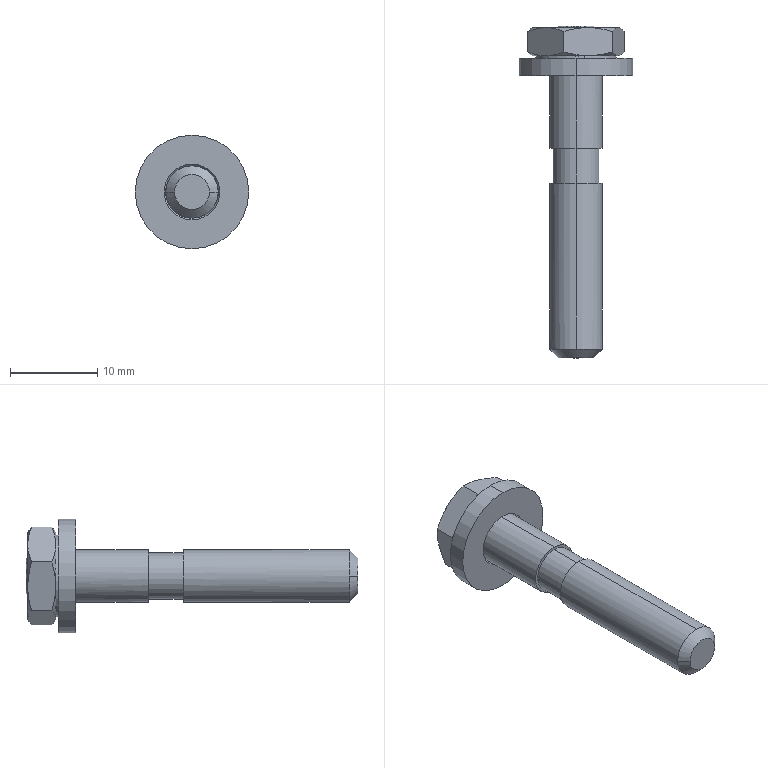Part | SolidWorks | features BaseBody 1 | 1 solid | 59 faces | box 13 x 38 x 13 mm | volume 1424 mm3 | cone 25 | cylinder 18 | plane 16 | commonest cylinder face diameters 6 x6 6.5 x3 9.3 x3 5.3 x2 6.4 x2 13 x2